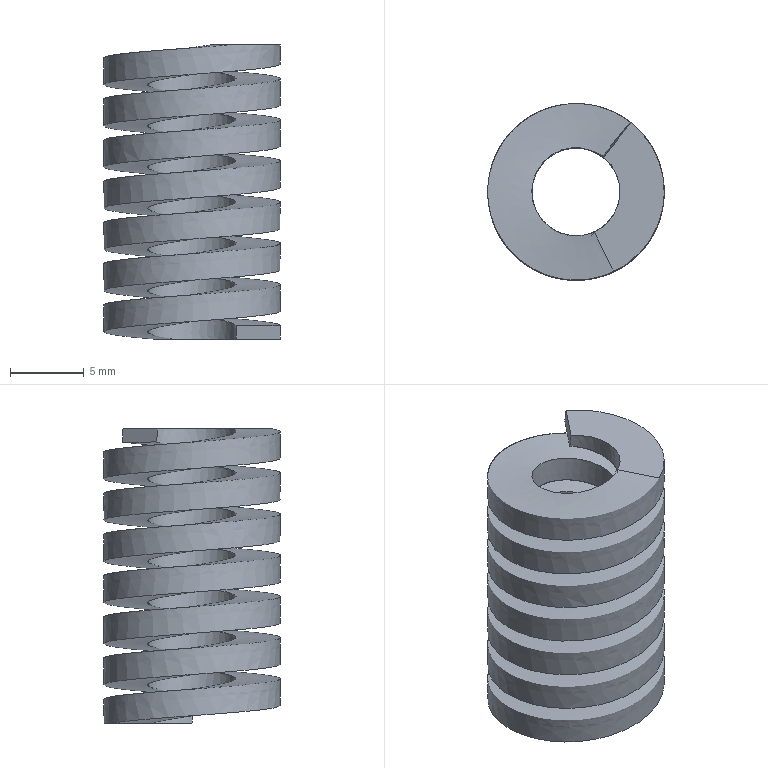Part | STEP file | E011204002 | 1 solid | 6 faces | volume 1089 mm3 | plane 4 | spline 2